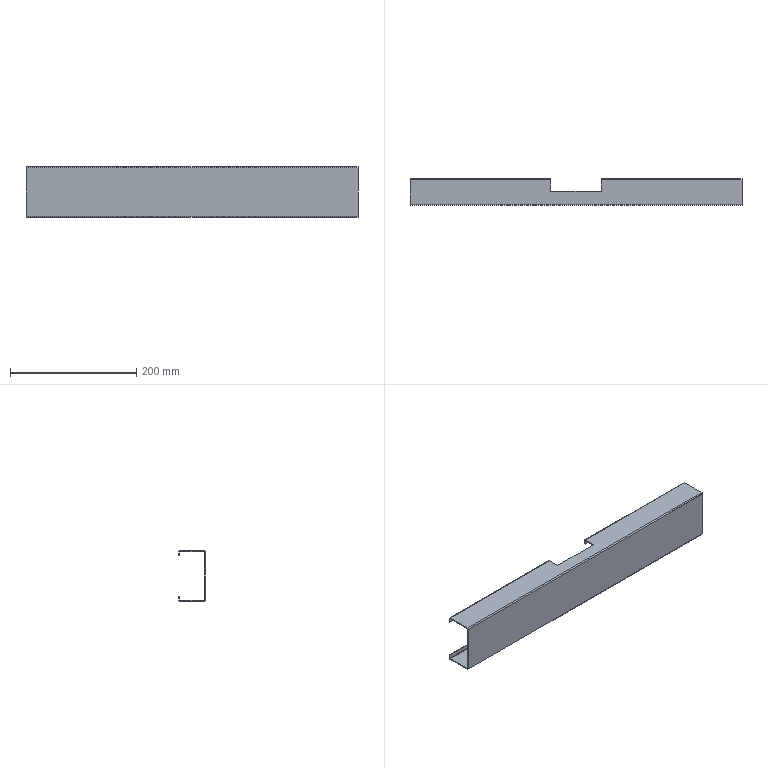Part | 1 solid | 62 faces | box 525 x 42 x 80 mm | volume 129478 mm3 | plane 50 | cylinder 12 | commonest cylinder face diameters 0.4 x6 3.4 x6
STEP:
#1=CARTESIAN_POINT('',(-40.,42.,38.3));
#2=VERTEX_POINT('',#1);
#3=CARTESIAN_POINT('',(-40.,42.,32.));
#4=VERTEX_POINT('',#3);
#5=CARTESIAN_POINT('',(-40.,42.,32.));
#6=DIRECTION('',(0.,0.,-1.));
#7=VECTOR('',#6,1000.);
#8=LINE('',#5,#7);
#9=EDGE_CURVE('',#2,#4,#8,.T.);
#10=ORIENTED_EDGE('',*,*,#9,.F.);
#11=CARTESIAN_POINT('',(-40.,40.5,38.3));
#12=VERTEX_POINT('',#11);
#13=CARTESIAN_POINT('',(-40.,42.,38.3));
#14=DIRECTION('',(0.,-1.,0.));
#15=VECTOR('',#14,1000.);
#16=LINE('',#13,#15);
#17=EDGE_CURVE('',#2,#12,#16,.T.);
#18=ORIENTED_EDGE('',*,*,#17,.T.);
#19=CARTESIAN_POINT('',(-40.,40.5,32.));
#20=VERTEX_POINT('',#19);
#21=CARTESIAN_POINT('',(-40.,40.5,32.));
#22=DIRECTION('',(0.,0.,-1.));
#23=VECTOR('',#22,1000.);
#24=LINE('',#21,#23);
#25=EDGE_CURVE('',#12,#20,#24,.T.);
#26=ORIENTED_EDGE('',*,*,#25,.T.);
#27=CARTESIAN_POINT('',(-40.,42.,32.));
#28=DIRECTION('',(0.,1.,0.));
#29=VECTOR('',#28,1000.);
#30=LINE('',#27,#29);
#31=EDGE_CURVE('',#20,#4,#30,.T.);
#32=ORIENTED_EDGE('',*,*,#31,.T.);
#33=EDGE_LOOP('',(#10,#18,#26,#32));
#34=FACE_OUTER_BOUND('',#33,.T.);
#35=CARTESIAN_POINT('',(-40.,62.,-40.));
#36=DIRECTION('',(-1.,0.,0.));
#37=DIRECTION('',(0.,0.,1.));
#38=AXIS2_PLACEMENT_3D('',#35,#36,#37);
#39=PLANE('',#38);
#40=ADVANCED_FACE('',(#34),#39,.F.);
#41=CARTESIAN_POINT('',(-40.,22.,38.5));
#42=VERTEX_POINT('',#41);
#43=CARTESIAN_POINT('',(-40.,40.3,38.5));
#44=VERTEX_POINT('',#43);
#45=CARTESIAN_POINT('',(-40.,42.,38.5));
#46=DIRECTION('',(0.,1.,0.));
#47=VECTOR('',#46,1000.);
#48=LINE('',#45,#47);
#49=EDGE_CURVE('',#42,#44,#48,.T.);
#50=ORIENTED_EDGE('',*,*,#49,.T.);
#51=CARTESIAN_POINT('',(-40.,40.3,40.));
#52=VERTEX_POINT('',#51);
#53=CARTESIAN_POINT('',(-40.,40.3,38.5));
#54=DIRECTION('',(0.,0.,1.));
#55=VECTOR('',#54,1000.);
#56=LINE('',#53,#55);
#57=EDGE_CURVE('',#44,#52,#56,.T.);
#58=ORIENTED_EDGE('',*,*,#57,.T.);
#59=CARTESIAN_POINT('',(-40.,22.,40.));
#60=VERTEX_POINT('',#59);
#61=CARTESIAN_POINT('',(-40.,42.,40.));
#62=DIRECTION('',(0.,1.,0.));
#63=VECTOR('',#62,1000.);
#64=LINE('',#61,#63);
#65=EDGE_CURVE('',#60,#52,#64,.T.);
#66=ORIENTED_EDGE('',*,*,#65,.F.);
#67=CARTESIAN_POINT('',(-40.,22.,-40.));
#68=DIRECTION('',(0.,0.,1.));
#69=VECTOR('',#68,1000.);
#70=LINE('',#67,#69);
#71=EDGE_CURVE('',#42,#60,#70,.T.);
#72=ORIENTED_EDGE('',*,*,#71,.F.);
#73=EDGE_LOOP('',(#50,#58,#66,#72));
#74=FACE_OUTER_BOUND('',#73,.T.);
#75=CARTESIAN_POINT('',(-40.,62.,-40.));
#76=DIRECTION('',(-1.,0.,0.));
#77=DIRECTION('',(0.,0.,1.));
#78=AXIS2_PLACEMENT_3D('',#75,#76,#77);
#79=PLANE('',#78);
#80=ADVANCED_FACE('',(#74),#79,.F.);
#81=CARTESIAN_POINT('',(40.,40.5,32.));
#82=VERTEX_POINT('',#81);
#83=CARTESIAN_POINT('',(40.,40.5,38.3));
#84=VERTEX_POINT('',#83);
#85=CARTESIAN_POINT('',(40.,40.5,32.));
#86=DIRECTION('',(0.,0.,1.));
#87=VECTOR('',#86,1000.);
#88=LINE('',#85,#87);
#89=EDGE_CURVE('',#82,#84,#88,.T.);
#90=ORIENTED_EDGE('',*,*,#89,.T.);
#91=CARTESIAN_POINT('',(40.,42.,38.3));
#92=VERTEX_POINT('',#91);
#93=CARTESIAN_POINT('',(40.,40.5,38.3));
#94=DIRECTION('',(0.,1.,0.));
#95=VECTOR('',#94,1000.);
#96=LINE('',#93,#95);
#97=EDGE_CURVE('',#84,#92,#96,.T.);
#98=ORIENTED_EDGE('',*,*,#97,.T.);
#99=CARTESIAN_POINT('',(40.,42.,32.));
#100=VERTEX_POINT('',#99);
#101=CARTESIAN_POINT('',(40.,42.,32.));
#102=DIRECTION('',(0.,0.,1.));
#103=VECTOR('',#102,1000.);
#104=LINE('',#101,#103);
#105=EDGE_CURVE('',#100,#92,#104,.T.);
#106=ORIENTED_EDGE('',*,*,#105,.F.);
#107=CARTESIAN_POINT('',(40.,42.,32.));
#108=DIRECTION('',(0.,-1.,0.));
#109=VECTOR('',#108,1000.);
#110=LINE('',#107,#109);
#111=EDGE_CURVE('',#100,#82,#110,.T.);
#112=ORIENTED_EDGE('',*,*,#111,.T.);
#113=EDGE_LOOP('',(#90,#98,#106,#112));
#114=FACE_OUTER_BOUND('',#113,.T.);
#115=CARTESIAN_POINT('',(40.,62.,-40.));
#116=DIRECTION('',(1.,0.,0.));
#117=DIRECTION('',(0.,0.,-1.));
#118=AXIS2_PLACEMENT_3D('',#115,#116,#117);
#119=PLANE('',#118);
#120=ADVANCED_FACE('',(#114),#119,.F.);
#121=CARTESIAN_POINT('',(40.,40.3,40.));
#122=VERTEX_POINT('',#121);
#123=CARTESIAN_POINT('',(40.,22.,40.));
#124=VERTEX_POINT('',#123);
#125=CARTESIAN_POINT('',(40.,42.,40.));
#126=DIRECTION('',(0.,-1.,0.));
#127=VECTOR('',#126,1000.);
#128=LINE('',#125,#127);
#129=EDGE_CURVE('',#122,#124,#128,.T.);
#130=ORIENTED_EDGE('',*,*,#129,.F.);
#131=CARTESIAN_POINT('',(40.,40.3,38.5));
#132=VERTEX_POINT('',#131);
#133=CARTESIAN_POINT('',(40.,40.3,40.));
#134=DIRECTION('',(0.,0.,-1.));
#135=VECTOR('',#134,1000.);
#136=LINE('',#133,#135);
#137=EDGE_CURVE('',#122,#132,#136,.T.);
#138=ORIENTED_EDGE('',*,*,#137,.T.);
#139=CARTESIAN_POINT('',(40.,22.,38.5));
#140=VERTEX_POINT('',#139);
#141=CARTESIAN_POINT('',(40.,42.,38.5));
#142=DIRECTION('',(0.,-1.,0.));
#143=VECTOR('',#142,1000.);
#144=LINE('',#141,#143);
#145=EDGE_CURVE('',#132,#140,#144,.T.);
#146=ORIENTED_EDGE('',*,*,#145,.T.);
#147=CARTESIAN_POINT('',(40.,22.,-40.));
#148=DIRECTION('',(0.,0.,1.));
#149=VECTOR('',#148,1000.);
#150=LINE('',#147,#149);
#151=EDGE_CURVE('',#140,#124,#150,.T.);
#152=ORIENTED_EDGE('',*,*,#151,.T.);
#153=EDGE_LOOP('',(#130,#138,#146,#152));
#154=FACE_OUTER_BOUND('',#153,.T.);
#155=CARTESIAN_POINT('',(40.,62.,-40.));
#156=DIRECTION('',(1.,0.,0.));
#157=DIRECTION('',(0.,0.,-1.));
#158=AXIS2_PLACEMENT_3D('',#155,#156,#157);
#159=PLANE('',#158);
#160=ADVANCED_FACE('',(#154),#159,.F.);
#161=CARTESIAN_POINT('',(-40.,40.5,-32.));
#162=VERTEX_POINT('',#161);
#163=CARTESIAN_POINT('',(-40.,40.5,-38.3));
#164=VERTEX_POINT('',#163);
#165=CARTESIAN_POINT('',(-40.,40.5,-40.));
#166=DIRECTION('',(0.,0.,-1.));
#167=VECTOR('',#166,1000.);
#168=LINE('',#165,#167);
#169=EDGE_CURVE('',#162,#164,#168,.T.);
#170=ORIENTED_EDGE('',*,*,#169,.T.);
#171=CARTESIAN_POINT('',(-40.,42.,-38.3));
#172=VERTEX_POINT('',#171);
#173=CARTESIAN_POINT('',(-40.,40.5,-38.3));
#174=DIRECTION('',(0.,1.,0.));
#175=VECTOR('',#174,1000.);
#176=LINE('',#173,#175);
#177=EDGE_CURVE('',#164,#172,#176,.T.);
#178=ORIENTED_EDGE('',*,*,#177,.T.);
#179=CARTESIAN_POINT('',(-40.,42.,-32.));
#180=VERTEX_POINT('',#179);
#181=CARTESIAN_POINT('',(-40.,42.,-40.));
#182=DIRECTION('',(0.,0.,-1.));
#183=VECTOR('',#182,1000.);
#184=LINE('',#181,#183);
#185=EDGE_CURVE('',#180,#172,#184,.T.);
#186=ORIENTED_EDGE('',*,*,#185,.F.);
#187=CARTESIAN_POINT('',(-40.,40.5,-32.));
#188=DIRECTION('',(0.,-1.,0.));
#189=VECTOR('',#188,1000.);
#190=LINE('',#187,#189);
#191=EDGE_CURVE('',#180,#162,#190,.T.);
#192=ORIENTED_EDGE('',*,*,#191,.T.);
#193=EDGE_LOOP('',(#170,#178,#186,#192));
#194=FACE_OUTER_BOUND('',#193,.T.);
#195=CARTESIAN_POINT('',(-40.,62.,-40.));
#196=DIRECTION('',(-1.,0.,0.));
#197=DIRECTION('',(0.,0.,1.));
#198=AXIS2_PLACEMENT_3D('',#195,#196,#197);
#199=PLANE('',#198);
#200=ADVANCED_FACE('',(#194),#199,.F.);
#201=CARTESIAN_POINT('',(-40.,40.3,-40.));
#202=VERTEX_POINT('',#201);
#203=CARTESIAN_POINT('',(-40.,22.,-40.));
#204=VERTEX_POINT('',#203);
#205=CARTESIAN_POINT('',(-40.,62.,-40.));
#206=DIRECTION('',(0.,-1.,0.));
#207=VECTOR('',#206,1000.);
#208=LINE('',#205,#207);
#209=EDGE_CURVE('',#202,#204,#208,.T.);
#210=ORIENTED_EDGE('',*,*,#209,.F.);
#211=CARTESIAN_POINT('',(-40.,40.3,-38.5));
#212=VERTEX_POINT('',#211);
#213=CARTESIAN_POINT('',(-40.,40.3,-40.));
#214=DIRECTION('',(0.,0.,1.));
#215=VECTOR('',#214,1000.);
#216=LINE('',#213,#215);
#217=EDGE_CURVE('',#202,#212,#216,.T.);
#218=ORIENTED_EDGE('',*,*,#217,.T.);
#219=CARTESIAN_POINT('',(-40.,22.,-38.5));
#220=VERTEX_POINT('',#219);
#221=CARTESIAN_POINT('',(-40.,0.,-38.5));
#222=DIRECTION('',(0.,-1.,0.));
#223=VECTOR('',#222,1000.);
#224=LINE('',#221,#223);
#225=EDGE_CURVE('',#212,#220,#224,.T.);
#226=ORIENTED_EDGE('',*,*,#225,.T.);
#227=CARTESIAN_POINT('',(-40.,22.,-40.));
#228=DIRECTION('',(0.,0.,1.));
#229=VECTOR('',#228,1000.);
#230=LINE('',#227,#229);
#231=EDGE_CURVE('',#204,#220,#230,.T.);
#232=ORIENTED_EDGE('',*,*,#231,.F.);
#233=EDGE_LOOP('',(#210,#218,#226,#232));
#234=FACE_OUTER_BOUND('',#233,.T.);
#235=CARTESIAN_POINT('',(-40.,62.,-40.));
#236=DIRECTION('',(-1.,0.,0.));
#237=DIRECTION('',(0.,0.,1.));
#238=AXIS2_PLACEMENT_3D('',#235,#236,#237);
#239=PLANE('',#238);
#240=ADVANCED_FACE('',(#234),#239,.F.);
#241=CARTESIAN_POINT('',(40.,42.,-38.3));
#242=VERTEX_POINT('',#241);
#243=CARTESIAN_POINT('',(40.,42.,-32.));
#244=VERTEX_POINT('',#243);
#245=CARTESIAN_POINT('',(40.,42.,-40.));
#246=DIRECTION('',(0.,0.,1.));
#247=VECTOR('',#246,1000.);
#248=LINE('',#245,#247);
#249=EDGE_CURVE('',#242,#244,#248,.T.);
#250=ORIENTED_EDGE('',*,*,#249,.F.);
#251=CARTESIAN_POINT('',(40.,40.5,-38.3));
#252=VERTEX_POINT('',#251);
#253=CARTESIAN_POINT('',(40.,42.,-38.3));
#254=DIRECTION('',(0.,-1.,0.));
#255=VECTOR('',#254,1000.);
#256=LINE('',#253,#255);
#257=EDGE_CURVE('',#242,#252,#256,.T.);
#258=ORIENTED_EDGE('',*,*,#257,.T.);
#259=CARTESIAN_POINT('',(40.,40.5,-32.));
#260=VERTEX_POINT('',#259);
#261=CARTESIAN_POINT('',(40.,40.5,-40.));
#262=DIRECTION('',(0.,0.,1.));
#263=VECTOR('',#262,1000.);
#264=LINE('',#261,#263);
#265=EDGE_CURVE('',#252,#260,#264,.T.);
#266=ORIENTED_EDGE('',*,*,#265,.T.);
#267=CARTESIAN_POINT('',(40.,40.5,-32.));
#268=DIRECTION('',(0.,1.,0.));
#269=VECTOR('',#268,1000.);
#270=LINE('',#267,#269);
#271=EDGE_CURVE('',#260,#244,#270,.T.);
#272=ORIENTED_EDGE('',*,*,#271,.T.);
#273=EDGE_LOOP('',(#250,#258,#266,#272));
#274=FACE_OUTER_BOUND('',#273,.T.);
#275=CARTESIAN_POINT('',(40.,62.,-40.));
#276=DIRECTION('',(1.,0.,0.));
#277=DIRECTION('',(0.,0.,-1.));
#278=AXIS2_PLACEMENT_3D('',#275,#276,#277);
#279=PLANE('',#278);
#280=ADVANCED_FACE('',(#274),#279,.F.);
#281=CARTESIAN_POINT('',(40.,22.,-38.5));
#282=VERTEX_POINT('',#281);
#283=CARTESIAN_POINT('',(40.,40.3,-38.5));
#284=VERTEX_POINT('',#283);
#285=CARTESIAN_POINT('',(40.,0.,-38.5));
#286=DIRECTION('',(0.,1.,0.));
#287=VECTOR('',#286,1000.);
#288=LINE('',#285,#287);
#289=EDGE_CURVE('',#282,#284,#288,.T.);
#290=ORIENTED_EDGE('',*,*,#289,.T.);
#291=CARTESIAN_POINT('',(40.,40.3,-40.));
#292=VERTEX_POINT('',#291);
#293=CARTESIAN_POINT('',(40.,40.3,-38.5));
#294=DIRECTION('',(0.,0.,-1.));
#295=VECTOR('',#294,1000.);
#296=LINE('',#293,#295);
#297=EDGE_CURVE('',#284,#292,#296,.T.);
#298=ORIENTED_EDGE('',*,*,#297,.T.);
#299=CARTESIAN_POINT('',(40.,22.,-40.));
#300=VERTEX_POINT('',#299);
#301=CARTESIAN_POINT('',(40.,62.,-40.));
#302=DIRECTION('',(0.,1.,0.));
#303=VECTOR('',#302,1000.);
#304=LINE('',#301,#303);
#305=EDGE_CURVE('',#300,#292,#304,.T.);
#306=ORIENTED_EDGE('',*,*,#305,.F.);
#307=CARTESIAN_POINT('',(40.,22.,-40.));
#308=DIRECTION('',(0.,0.,1.));
#309=VECTOR('',#308,1000.);
#310=LINE('',#307,#309);
#311=EDGE_CURVE('',#300,#282,#310,.T.);
#312=ORIENTED_EDGE('',*,*,#311,.T.);
#313=EDGE_LOOP('',(#290,#298,#306,#312));
#314=FACE_OUTER_BOUND('',#313,.T.);
#315=CARTESIAN_POINT('',(40.,62.,-40.));
#316=DIRECTION('',(1.,0.,0.));
#317=DIRECTION('',(0.,0.,-1.));
#318=AXIS2_PLACEMENT_3D('',#315,#316,#317);
#319=PLANE('',#318);
#320=ADVANCED_FACE('',(#314),#319,.F.);
#321=CARTESIAN_POINT('',(262.5,42.,-38.3));
#322=VERTEX_POINT('',#321);
#323=CARTESIAN_POINT('',(262.5,42.,-38.3));
#324=DIRECTION('',(-1.,0.,0.));
#325=VECTOR('',#324,1000.);
#326=LINE('',#323,#325);
#327=EDGE_CURVE('',#322,#242,#326,.T.);
#328=ORIENTED_EDGE('',*,*,#327,.T.);
#329=ORIENTED_EDGE('',*,*,#249,.T.);
#330=CARTESIAN_POINT('',(262.5,42.,-32.));
#331=VERTEX_POINT('',#330);
#332=CARTESIAN_POINT('',(262.5,42.,-32.));
#333=DIRECTION('',(-1.,0.,0.));
#334=VECTOR('',#333,1000.);
#335=LINE('',#332,#334);
#336=EDGE_CURVE('',#331,#244,#335,.T.);
#337=ORIENTED_EDGE('',*,*,#336,.F.);
#338=CARTESIAN_POINT('',(262.5,42.,-40.));
#339=DIRECTION('',(0.,0.,1.));
#340=VECTOR('',#339,1000.);
#341=LINE('',#338,#340);
#342=EDGE_CURVE('',#322,#331,#341,.T.);
#343=ORIENTED_EDGE('',*,*,#342,.F.);
#344=EDGE_LOOP('',(#328,#329,#337,#343));
#345=FACE_OUTER_BOUND('',#344,.T.);
#346=CARTESIAN_POINT('',(262.5,42.,-40.));
#347=DIRECTION('',(0.,-1.,0.));
#348=DIRECTION('',(0.,0.,-1.));
#349=AXIS2_PLACEMENT_3D('',#346,#347,#348);
#350=PLANE('',#349);
#351=ADVANCED_FACE('',(#345),#350,.F.);
#352=ORIENTED_EDGE('',*,*,#271,.F.);
#353=CARTESIAN_POINT('',(262.5,40.5,-32.));
#354=VERTEX_POINT('',#353);
#355=CARTESIAN_POINT('',(262.5,40.5,-32.));
#356=DIRECTION('',(-1.,0.,0.));
#357=VECTOR('',#356,1000.);
#358=LINE('',#355,#357);
#359=EDGE_CURVE('',#354,#260,#358,.T.);
#360=ORIENTED_EDGE('',*,*,#359,.F.);
#361=CARTESIAN_POINT('',(262.5,40.5,-32.));
#362=DIRECTION('',(0.,1.,0.));
#363=VECTOR('',#362,1000.);
#364=LINE('',#361,#363);
#365=EDGE_CURVE('',#354,#331,#364,.T.);
#366=ORIENTED_EDGE('',*,*,#365,.T.);
#367=ORIENTED_EDGE('',*,*,#336,.T.);
#368=EDGE_LOOP('',(#352,#360,#366,#367));
#369=FACE_OUTER_BOUND('',#368,.T.);
#370=CARTESIAN_POINT('',(262.5,40.5,-32.));
#371=DIRECTION('',(0.,0.,1.));
#372=DIRECTION('',(1.,0.,0.));
#373=AXIS2_PLACEMENT_3D('',#370,#371,#372);
#374=PLANE('',#373);
#375=ADVANCED_FACE('',(#369),#374,.T.);
#376=ORIENTED_EDGE('',*,*,#265,.F.);
#377=CARTESIAN_POINT('',(262.5,40.5,-38.3));
#378=VERTEX_POINT('',#377);
#379=CARTESIAN_POINT('',(262.5,40.5,-38.3));
#380=DIRECTION('',(-1.,0.,0.));
#381=VECTOR('',#380,1000.);
#382=LINE('',#379,#381);
#383=EDGE_CURVE('',#378,#252,#382,.T.);
#384=ORIENTED_EDGE('',*,*,#383,.F.);
#385=CARTESIAN_POINT('',(262.5,40.5,-40.));
#386=DIRECTION('',(0.,0.,1.));
#387=VECTOR('',#386,1000.);
#388=LINE('',#385,#387);
#389=EDGE_CURVE('',#378,#354,#388,.T.);
#390=ORIENTED_EDGE('',*,*,#389,.T.);
#391=ORIENTED_EDGE('',*,*,#359,.T.);
#392=EDGE_LOOP('',(#376,#384,#390,#391));
#393=FACE_OUTER_BOUND('',#392,.T.);
#394=CARTESIAN_POINT('',(262.5,40.5,-40.));
#395=DIRECTION('',(0.,-1.,0.));
#396=DIRECTION('',(0.,0.,-1.));
#397=AXIS2_PLACEMENT_3D('',#394,#395,#396);
#398=PLANE('',#397);
#399=ADVANCED_FACE('',(#393),#398,.T.);
#400=CARTESIAN_POINT('',(40.,40.3,-38.3));
#401=DIRECTION('',(1.,0.,0.));
#402=DIRECTION('',(0.,0.,-1.));
#403=AXIS2_PLACEMENT_3D('',#400,#401,#402);
#404=CIRCLE('',#403,0.2);
#405=EDGE_CURVE('',#284,#252,#404,.T.);
#406=ORIENTED_EDGE('',*,*,#405,.F.);
#407=CARTESIAN_POINT('',(262.5,40.3,-38.5));
#408=VERTEX_POINT('',#407);
#409=CARTESIAN_POINT('',(262.5,40.3,-38.5));
#410=DIRECTION('',(-1.,0.,0.));
#411=VECTOR('',#410,1000.);
#412=LINE('',#409,#411);
#413=EDGE_CURVE('',#408,#284,#412,.T.);
#414=ORIENTED_EDGE('',*,*,#413,.F.);
#415=CARTESIAN_POINT('',(262.5,40.3,-38.3));
#416=DIRECTION('',(1.,0.,0.));
#417=DIRECTION('',(0.,0.,-1.));
#418=AXIS2_PLACEMENT_3D('',#415,#416,#417);
#419=CIRCLE('',#418,0.2);
#420=EDGE_CURVE('',#408,#378,#419,.T.);
#421=ORIENTED_EDGE('',*,*,#420,.T.);
#422=ORIENTED_EDGE('',*,*,#383,.T.);
#423=EDGE_LOOP('',(#406,#414,#421,#422));
#424=FACE_OUTER_BOUND('',#423,.T.);
#425=CARTESIAN_POINT('',(262.5,40.3,-38.3));
#426=DIRECTION('',(-1.,0.,0.));
#427=DIRECTION('',(0.,0.,1.));
#428=AXIS2_PLACEMENT_3D('',#425,#426,#427);
#429=CYLINDRICAL_SURFACE('',#428,0.2);
#430=ADVANCED_FACE('',(#424),#429,.F.);
#431=CARTESIAN_POINT('',(40.,40.3,38.3));
#432=DIRECTION('',(1.,0.,0.));
#433=DIRECTION('',(0.,0.,-1.));
#434=AXIS2_PLACEMENT_3D('',#431,#432,#433);
#435=CIRCLE('',#434,0.2);
#436=EDGE_CURVE('',#84,#132,#435,.T.);
#437=ORIENTED_EDGE('',*,*,#436,.F.);
#438=CARTESIAN_POINT('',(262.5,40.5,38.3));
#439=VERTEX_POINT('',#438);
#440=CARTESIAN_POINT('',(262.5,40.5,38.3));
#441=DIRECTION('',(-1.,0.,0.));
#442=VECTOR('',#441,1000.);
#443=LINE('',#440,#442);
#444=EDGE_CURVE('',#439,#84,#443,.T.);
#445=ORIENTED_EDGE('',*,*,#444,.F.);
#446=CARTESIAN_POINT('',(262.5,40.3,38.5));
#447=VERTEX_POINT('',#446);
#448=CARTESIAN_POINT('',(262.5,40.3,38.3));
#449=DIRECTION('',(1.,0.,0.));
#450=DIRECTION('',(0.,0.,-1.));
#451=AXIS2_PLACEMENT_3D('',#448,#449,#450);
#452=CIRCLE('',#451,0.2);
#453=EDGE_CURVE('',#439,#447,#452,.T.);
#454=ORIENTED_EDGE('',*,*,#453,.T.);
#455=CARTESIAN_POINT('',(262.5,40.3,38.5));
#456=DIRECTION('',(-1.,0.,0.));
#457=VECTOR('',#456,1000.);
#458=LINE('',#455,#457);
#459=EDGE_CURVE('',#447,#132,#458,.T.);
#460=ORIENTED_EDGE('',*,*,#459,.T.);
#461=EDGE_LOOP('',(#437,#445,#454,#460));
#462=FACE_OUTER_BOUND('',#461,.T.);
#463=CARTESIAN_POINT('',(262.5,40.3,38.3));
#464=DIRECTION('',(-1.,0.,0.));
#465=DIRECTION('',(0.,0.,1.));
#466=AXIS2_PLACEMENT_3D('',#463,#464,#465);
#467=CYLINDRICAL_SURFACE('',#466,0.2);
#468=ADVANCED_FACE('',(#462),#467,.F.);
#469=ORIENTED_EDGE('',*,*,#89,.F.);
#470=CARTESIAN_POINT('',(262.5,40.5,32.));
#471=VERTEX_POINT('',#470);
#472=CARTESIAN_POINT('',(262.5,40.5,32.));
#473=DIRECTION('',(-1.,0.,0.));
#474=VECTOR('',#473,1000.);
#475=LINE('',#472,#474);
#476=EDGE_CURVE('',#471,#82,#475,.T.);
#477=ORIENTED_EDGE('',*,*,#476,.F.);
#478=CARTESIAN_POINT('',(262.5,40.5,32.));
#479=DIRECTION('',(0.,0.,1.));
#480=VECTOR('',#479,1000.);
#481=LINE('',#478,#480);
#482=EDGE_CURVE('',#471,#439,#481,.T.);
#483=ORIENTED_EDGE('',*,*,#482,.T.);
#484=ORIENTED_EDGE('',*,*,#444,.T.);
#485=EDGE_LOOP('',(#469,#477,#483,#484));
#486=FACE_OUTER_BOUND('',#485,.T.);
#487=CARTESIAN_POINT('',(262.5,40.5,32.));
#488=DIRECTION('',(0.,-1.,0.));
#489=DIRECTION('',(0.,0.,-1.));
#490=AXIS2_PLACEMENT_3D('',#487,#488,#489);
#491=PLANE('',#490);
#492=ADVANCED_FACE('',(#486),#491,.T.);
#493=ORIENTED_EDGE('',*,*,#111,.F.);
#494=CARTESIAN_POINT('',(262.5,42.,32.));
#495=VERTEX_POINT('',#494);
#496=CARTESIAN_POINT('',(262.5,42.,32.));
#497=DIRECTION('',(-1.,0.,0.));
#498=VECTOR('',#497,1000.);
#499=LINE('',#496,#498);
#500=EDGE_CURVE('',#495,#100,#499,.T.);
#501=ORIENTED_EDGE('',*,*,#500,.F.);
#502=CARTESIAN_POINT('',(262.5,42.,32.));
#503=DIRECTION('',(0.,-1.,0.));
#504=VECTOR('',#503,1000.);
#505=LINE('',#502,#504);
#506=EDGE_CURVE('',#495,#471,#505,.T.);
#507=ORIENTED_EDGE('',*,*,#506,.T.);
#508=ORIENTED_EDGE('',*,*,#476,.T.);
#509=EDGE_LOOP('',(#493,#501,#507,#508));
#510=FACE_OUTER_BOUND('',#509,.T.);
#511=CARTESIAN_POINT('',(262.5,42.,32.));
#512=DIRECTION('',(0.,0.,-1.));
#513=DIRECTION('',(-1.,0.,0.));
#514=AXIS2_PLACEMENT_3D('',#511,#512,#513);
#515=PLANE('',#514);
#516=ADVANCED_FACE('',(#510),#515,.T.);
#517=ORIENTED_EDGE('',*,*,#500,.T.);
#518=ORIENTED_EDGE('',*,*,#105,.T.);
#519=CARTESIAN_POINT('',(262.5,42.,38.3));
#520=VERTEX_POINT('',#519);
#521=CARTESIAN_POINT('',(262.5,42.,38.3));
#522=DIRECTION('',(-1.,0.,0.));
#523=VECTOR('',#522,1000.);
#524=LINE('',#521,#523);
#525=EDGE_CURVE('',#520,#92,#524,.T.);
#526=ORIENTED_EDGE('',*,*,#525,.F.);
#527=CARTESIAN_POINT('',(262.5,42.,32.));
#528=DIRECTION('',(0.,0.,1.));
#529=VECTOR('',#528,1000.);
#530=LINE('',#527,#529);
#531=EDGE_CURVE('',#495,#520,#530,.T.);
#532=ORIENTED_EDGE('',*,*,#531,.F.);
#533=EDGE_LOOP('',(#517,#518,#526,#532));
#534=FACE_OUTER_BOUND('',#533,.T.);
#535=CARTESIAN_POINT('',(262.5,42.,32.));
#536=DIRECTION('',(0.,-1.,0.));
#537=DIRECTION('',(0.,0.,-1.));
#538=AXIS2_PLACEMENT_3D('',#535,#536,#537);
#539=PLANE('',#538);
#540=ADVANCED_FACE('',(#534),#539,.F.);
#541=ORIENTED_EDGE('',*,*,#525,.T.);
#542=CARTESIAN_POINT('',(40.,40.3,38.3));
#543=DIRECTION('',(1.,0.,0.));
#544=DIRECTION('',(0.,0.,-1.));
#545=AXIS2_PLACEMENT_3D('',#542,#543,#544);
#546=CIRCLE('',#545,1.7);
#547=EDGE_CURVE('',#92,#122,#546,.T.);
#548=ORIENTED_EDGE('',*,*,#547,.T.);
#549=CARTESIAN_POINT('',(262.5,40.3,40.));
#550=VERTEX_POINT('',#549);
#551=CARTESIAN_POINT('',(262.5,40.3,40.));
#552=DIRECTION('',(-1.,0.,0.));
#553=VECTOR('',#552,1000.);
#554=LINE('',#551,#553);
#555=EDGE_CURVE('',#550,#122,#554,.T.);
#556=ORIENTED_EDGE('',*,*,#555,.F.);
#557=CARTESIAN_POINT('',(262.5,40.3,38.3));
#558=DIRECTION('',(1.,0.,0.));
#559=DIRECTION('',(0.,0.,1.));
#560=AXIS2_PLACEMENT_3D('',#557,#558,#559);
#561=CIRCLE('',#560,1.7);
#562=EDGE_CURVE('',#520,#550,#561,.T.);
#563=ORIENTED_EDGE('',*,*,#562,.F.);
#564=EDGE_LOOP('',(#541,#548,#556,#563));
#565=FACE_OUTER_BOUND('',#564,.T.);
#566=CARTESIAN_POINT('',(262.5,40.3,38.3));
#567=DIRECTION('',(-1.,0.,0.));
#568=DIRECTION('',(0.,0.,1.));
#569=AXIS2_PLACEMENT_3D('',#566,#567,#568);
#570=CYLINDRICAL_SURFACE('',#569,1.7);
#571=ADVANCED_FACE('',(#565),#570,.T.);
#572=CARTESIAN_POINT('',(262.5,40.3,-40.));
#573=VERTEX_POINT('',#572);
#574=CARTESIAN_POINT('',(262.5,40.3,-40.));
#575=DIRECTION('',(-1.,0.,0.));
#576=VECTOR('',#575,1000.);
#577=LINE('',#574,#576);
#578=EDGE_CURVE('',#573,#292,#577,.T.);
#579=ORIENTED_EDGE('',*,*,#578,.T.);
#580=CARTESIAN_POINT('',(40.,40.3,-38.3));
#581=DIRECTION('',(1.,0.,0.));
#582=DIRECTION('',(0.,0.,-1.));
#583=AXIS2_PLACEMENT_3D('',#580,#581,#582);
#584=CIRCLE('',#583,1.7);
#585=EDGE_CURVE('',#292,#242,#584,.T.);
#586=ORIENTED_EDGE('',*,*,#585,.T.);
#587=ORIENTED_EDGE('',*,*,#327,.F.);
#588=CARTESIAN_POINT('',(262.5,40.3,-38.3));
#589=DIRECTION('',(1.,0.,0.));
#590=DIRECTION('',(0.,0.,1.));
#591=AXIS2_PLACEMENT_3D('',#588,#589,#590);
#592=CIRCLE('',#591,1.7);
#593=EDGE_CURVE('',#573,#322,#592,.T.);
#594=ORIENTED_EDGE('',*,*,#593,.F.);
#595=EDGE_LOOP('',(#579,#586,#587,#594));
#596=FACE_OUTER_BOUND('',#595,.T.);
#597=CARTESIAN_POINT('',(262.5,40.3,-38.3));
#598=DIRECTION('',(-1.,0.,0.));
#599=DIRECTION('',(0.,0.,1.));
#600=AXIS2_PLACEMENT_3D('',#597,#598,#599);
#601=CYLINDRICAL_SURFACE('',#600,1.7);
#602=ADVANCED_FACE('',(#596),#601,.T.);
#603=CARTESIAN_POINT('',(262.5,42.,38.3));
#604=DIRECTION('',(0.,-1.,0.));
#605=VECTOR('',#604,1000.);
#606=LINE('',#603,#605);
#607=EDGE_CURVE('',#520,#439,#606,.T.);
#608=ORIENTED_EDGE('',*,*,#607,.F.);
#609=ORIENTED_EDGE('',*,*,#562,.T.);
#610=CARTESIAN_POINT('',(262.5,40.3,38.5));
#611=DIRECTION('',(0.,0.,1.));
#612=VECTOR('',#611,1000.);
#613=LINE('',#610,#612);
#614=EDGE_CURVE('',#447,#550,#613,.T.);
#615=ORIENTED_EDGE('',*,*,#614,.F.);
#616=ORIENTED_EDGE('',*,*,#453,.F.);
#617=EDGE_LOOP('',(#608,#609,#615,#616));
#618=FACE_OUTER_BOUND('',#617,.T.);
#619=CARTESIAN_POINT('',(262.5,42.,38.3));
#620=DIRECTION('',(1.,0.,0.));
#621=DIRECTION('',(0.,0.,-1.));
#622=AXIS2_PLACEMENT_3D('',#619,#620,#621);
#623=PLANE('',#622);
#624=ADVANCED_FACE('',(#618),#623,.T.);
#625=ORIENTED_EDGE('',*,*,#531,.T.);
#626=ORIENTED_EDGE('',*,*,#607,.T.);
#627=ORIENTED_EDGE('',*,*,#482,.F.);
#628=ORIENTED_EDGE('',*,*,#506,.F.);
#629=EDGE_LOOP('',(#625,#626,#627,#628));
#630=FACE_OUTER_BOUND('',#629,.T.);
#631=CARTESIAN_POINT('',(262.5,40.3,38.5));
#632=DIRECTION('',(1.,0.,0.));
#633=DIRECTION('',(0.,0.,-1.));
#634=AXIS2_PLACEMENT_3D('',#631,#632,#633);
#635=PLANE('',#634);
#636=ADVANCED_FACE('',(#630),#635,.T.);
#637=CARTESIAN_POINT('',(-262.5,40.3,40.));
#638=VERTEX_POINT('',#637);
#639=CARTESIAN_POINT('',(-262.5,40.3,38.5));
#640=VERTEX_POINT('',#639);
#641=CARTESIAN_POINT('',(-262.5,40.3,40.));
#642=DIRECTION('',(0.,0.,-1.));
#643=VECTOR('',#642,1000.);
#644=LINE('',#641,#643);
#645=EDGE_CURVE('',#638,#640,#644,.T.);
#646=ORIENTED_EDGE('',*,*,#645,.F.);
#647=CARTESIAN_POINT('',(-262.5,42.,38.3));
#648=VERTEX_POINT('',#647);
#649=CARTESIAN_POINT('',(-262.5,40.3,38.3));
#650=DIRECTION('',(1.,0.,0.));
#651=DIRECTION('',(0.,0.,1.));
#652=AXIS2_PLACEMENT_3D('',#649,#650,#651);
#653=CIRCLE('',#652,1.7);
#654=EDGE_CURVE('',#648,#638,#653,.T.);
#655=ORIENTED_EDGE('',*,*,#654,.F.);
#656=CARTESIAN_POINT('',(-262.5,40.5,38.3));
#657=VERTEX_POINT('',#656);
#658=CARTESIAN_POINT('',(-262.5,40.5,38.3));
#659=DIRECTION('',(0.,1.,0.));
#660=VECTOR('',#659,1000.);
#661=LINE('',#658,#660);
#662=EDGE_CURVE('',#657,#648,#661,.T.);
#663=ORIENTED_EDGE('',*,*,#662,.F.);
#664=CARTESIAN_POINT('',(-262.5,40.3,38.3));
#665=DIRECTION('',(1.,0.,0.));
#666=DIRECTION('',(0.,0.,-1.));
#667=AXIS2_PLACEMENT_3D('',#664,#665,#666);
#668=CIRCLE('',#667,0.2);
#669=EDGE_CURVE('',#657,#640,#668,.T.);
#670=ORIENTED_EDGE('',*,*,#669,.T.);
#671=EDGE_LOOP('',(#646,#655,#663,#670));
#672=FACE_OUTER_BOUND('',#671,.T.);
#673=CARTESIAN_POINT('',(-262.5,40.3,40.));
#674=DIRECTION('',(-1.,0.,0.));
#675=DIRECTION('',(0.,0.,1.));
#676=AXIS2_PLACEMENT_3D('',#673,#674,#675);
#677=PLANE('',#676);
#678=ADVANCED_FACE('',(#672),#677,.T.);
#679=CARTESIAN_POINT('',(-262.5,1.7,40.));
#680=VERTEX_POINT('',#679);
#681=CARTESIAN_POINT('',(-262.5,42.,40.));
#682=DIRECTION('',(0.,-1.,0.));
#683=VECTOR('',#682,1000.);
#684=LINE('',#681,#683);
#685=EDGE_CURVE('',#638,#680,#684,.T.);
#686=ORIENTED_EDGE('',*,*,#685,.F.);
#687=ORIENTED_EDGE('',*,*,#645,.T.);
#688=CARTESIAN_POINT('',(-262.5,1.7,38.5));
#689=VERTEX_POINT('',#688);
#690=CARTESIAN_POINT('',(-262.5,42.,38.5));
#691=DIRECTION('',(0.,-1.,0.));
#692=VECTOR('',#691,1000.);
#693=LINE('',#690,#692);
#694=EDGE_CURVE('',#640,#689,#693,.T.);
#695=ORIENTED_EDGE('',*,*,#694,.T.);
#696=CARTESIAN_POINT('',(-262.5,1.7,38.5));
#697=DIRECTION('',(0.,0.,1.));
#698=VECTOR('',#697,1000.);
#699=LINE('',#696,#698);
#700=EDGE_CURVE('',#689,#680,#699,.T.);
#701=ORIENTED_EDGE('',*,*,#700,.T.);
#702=EDGE_LOOP('',(#686,#687,#695,#701));
#703=FACE_OUTER_BOUND('',#702,.T.);
#704=CARTESIAN_POINT('',(-262.5,40.5,38.3));
#705=DIRECTION('',(-1.,0.,0.));
#706=DIRECTION('',(0.,0.,1.));
#707=AXIS2_PLACEMENT_3D('',#704,#705,#706);
#708=PLANE('',#707);
#709=ADVANCED_FACE('',(#703),#708,.T.);
#710=CARTESIAN_POINT('',(262.5,1.7,40.));
#711=VERTEX_POINT('',#710);
#712=CARTESIAN_POINT('',(262.5,1.7,38.5));
#713=VERTEX_POINT('',#712);
#714=CARTESIAN_POINT('',(262.5,1.7,40.));
#715=DIRECTION('',(0.,0.,-1.));
#716=VECTOR('',#715,1000.);
#717=LINE('',#714,#716);
#718=EDGE_CURVE('',#711,#713,#717,.T.);
#719=ORIENTED_EDGE('',*,*,#718,.F.);
#720=CARTESIAN_POINT('',(262.5,0.,38.3));
#721=VERTEX_POINT('',#720);
#722=CARTESIAN_POINT('',(262.5,1.7,38.3));
#723=DIRECTION('',(1.,0.,0.));
#724=DIRECTION('',(0.,0.,1.));
#725=AXIS2_PLACEMENT_3D('',#722,#723,#724);
#726=CIRCLE('',#725,1.7);
#727=EDGE_CURVE('',#711,#721,#726,.T.);
#728=ORIENTED_EDGE('',*,*,#727,.T.);
#729=CARTESIAN_POINT('',(262.5,1.5,38.3));
#730=VERTEX_POINT('',#729);
#731=CARTESIAN_POINT('',(262.5,1.5,38.3));
#732=DIRECTION('',(0.,-1.,0.));
#733=VECTOR('',#732,1000.);
#734=LINE('',#731,#733);
#735=EDGE_CURVE('',#730,#721,#734,.T.);
#736=ORIENTED_EDGE('',*,*,#735,.F.);
#737=CARTESIAN_POINT('',(262.5,1.7,38.3));
#738=DIRECTION('',(1.,0.,0.));
#739=DIRECTION('',(0.,0.,-1.));
#740=AXIS2_PLACEMENT_3D('',#737,#738,#739);
#741=CIRCLE('',#740,0.2);
#742=EDGE_CURVE('',#713,#730,#741,.T.);
#743=ORIENTED_EDGE('',*,*,#742,.F.);
#744=EDGE_LOOP('',(#719,#728,#736,#743));
#745=FACE_OUTER_BOUND('',#744,.T.);
#746=CARTESIAN_POINT('',(262.5,1.7,40.));
#747=DIRECTION('',(1.,0.,0.));
#748=DIRECTION('',(0.,0.,-1.));
#749=AXIS2_PLACEMENT_3D('',#746,#747,#748);
#750=PLANE('',#749);
#751=ADVANCED_FACE('',(#745),#750,.T.);
#752=CARTESIAN_POINT('',(262.5,42.,40.));
#753=DIRECTION('',(0.,-1.,0.));
#754=VECTOR('',#753,1000.);
#755=LINE('',#752,#754);
#756=EDGE_CURVE('',#550,#711,#755,.T.);
#757=ORIENTED_EDGE('',*,*,#756,.T.);
#758=ORIENTED_EDGE('',*,*,#718,.T.);
#759=CARTESIAN_POINT('',(262.5,42.,38.5));
#760=DIRECTION('',(0.,-1.,0.));
#761=VECTOR('',#760,1000.);
#762=LINE('',#759,#761);
#763=EDGE_CURVE('',#447,#713,#762,.T.);
#764=ORIENTED_EDGE('',*,*,#763,.F.);
#765=ORIENTED_EDGE('',*,*,#614,.T.);
#766=EDGE_LOOP('',(#757,#758,#764,#765));
#767=FACE_OUTER_BOUND('',#766,.T.);
#768=CARTESIAN_POINT('',(262.5,1.5,38.3));
#769=DIRECTION('',(1.,0.,0.));
#770=DIRECTION('',(0.,0.,-1.));
#771=AXIS2_PLACEMENT_3D('',#768,#769,#770);
#772=PLANE('',#771);
#773=ADVANCED_FACE('',(#767),#772,.T.);
#774=CARTESIAN_POINT('',(-262.5,0.,38.3));
#775=VERTEX_POINT('',#774);
#776=CARTESIAN_POINT('',(-262.5,1.5,38.3));
#777=VERTEX_POINT('',#776);
#778=CARTESIAN_POINT('',(-262.5,0.,38.3));
#779=DIRECTION('',(0.,1.,0.));
#780=VECTOR('',#779,1000.);
#781=LINE('',#778,#780);
#782=EDGE_CURVE('',#775,#777,#781,.T.);
#783=ORIENTED_EDGE('',*,*,#782,.F.);
#784=CARTESIAN_POINT('',(-262.5,1.7,38.3));
#785=DIRECTION('',(1.,0.,0.));
#786=DIRECTION('',(0.,0.,1.));
#787=AXIS2_PLACEMENT_3D('',#784,#785,#786);
#788=CIRCLE('',#787,1.7);
#789=EDGE_CURVE('',#680,#775,#788,.T.);
#790=ORIENTED_EDGE('',*,*,#789,.F.);
#791=ORIENTED_EDGE('',*,*,#700,.F.);
#792=CARTESIAN_POINT('',(-262.5,1.7,38.3));
#793=DIRECTION('',(1.,0.,0.));
#794=DIRECTION('',(0.,0.,-1.));
#795=AXIS2_PLACEMENT_3D('',#792,#793,#794);
#796=CIRCLE('',#795,0.2);
#797=EDGE_CURVE('',#689,#777,#796,.T.);
#798=ORIENTED_EDGE('',*,*,#797,.T.);
#799=EDGE_LOOP('',(#783,#790,#791,#798));
#800=FACE_OUTER_BOUND('',#799,.T.);
#801=CARTESIAN_POINT('',(-262.5,0.,38.3));
#802=DIRECTION('',(-1.,0.,0.));
#803=DIRECTION('',(0.,0.,1.));
#804=AXIS2_PLACEMENT_3D('',#801,#802,#803);
#805=PLANE('',#804);
#806=ADVANCED_FACE('',(#800),#805,.T.);
#807=CARTESIAN_POINT('',(-262.5,0.,-38.3));
#808=VERTEX_POINT('',#807);
#809=CARTESIAN_POINT('',(-262.5,0.,40.));
#810=DIRECTION('',(0.,0.,-1.));
#811=VECTOR('',#810,1000.);
#812=LINE('',#809,#811);
#813=EDGE_CURVE('',#775,#808,#812,.T.);
#814=ORIENTED_EDGE('',*,*,#813,.F.);
#815=ORIENTED_EDGE('',*,*,#782,.T.);
#816=CARTESIAN_POINT('',(-262.5,1.5,-38.3));
#817=VERTEX_POINT('',#816);
#818=CARTESIAN_POINT('',(-262.5,1.5,40.));
#819=DIRECTION('',(0.,0.,-1.));
#820=VECTOR('',#819,1000.);
#821=LINE('',#818,#820);
#822=EDGE_CURVE('',#777,#817,#821,.T.);
#823=ORIENTED_EDGE('',*,*,#822,.T.);
#824=CARTESIAN_POINT('',(-262.5,1.5,-38.3));
#825=DIRECTION('',(0.,-1.,0.));
#826=VECTOR('',#825,1000.);
#827=LINE('',#824,#826);
#828=EDGE_CURVE('',#817,#808,#827,.T.);
#829=ORIENTED_EDGE('',*,*,#828,.T.);
#830=EDGE_LOOP('',(#814,#815,#823,#829));
#831=FACE_OUTER_BOUND('',#830,.T.);
#832=CARTESIAN_POINT('',(-262.5,1.7,38.5));
#833=DIRECTION('',(-1.,0.,0.));
#834=DIRECTION('',(0.,0.,1.));
#835=AXIS2_PLACEMENT_3D('',#832,#833,#834);
#836=PLANE('',#835);
#837=ADVANCED_FACE('',(#831),#836,.T.);
#838=CARTESIAN_POINT('',(262.5,0.,-38.3));
#839=VERTEX_POINT('',#838);
#840=CARTESIAN_POINT('',(262.5,1.5,-38.3));
#841=VERTEX_POINT('',#840);
#842=CARTESIAN_POINT('',(262.5,0.,-38.3));
#843=DIRECTION('',(0.,1.,0.));
#844=VECTOR('',#843,1000.);
#845=LINE('',#842,#844);
#846=EDGE_CURVE('',#839,#841,#845,.T.);
#847=ORIENTED_EDGE('',*,*,#846,.F.);
#848=CARTESIAN_POINT('',(262.5,1.7,-40.));
#849=VERTEX_POINT('',#848);
#850=CARTESIAN_POINT('',(262.5,1.7,-38.3));
#851=DIRECTION('',(1.,0.,0.));
#852=DIRECTION('',(0.,0.,1.));
#853=AXIS2_PLACEMENT_3D('',#850,#851,#852);
#854=CIRCLE('',#853,1.7);
#855=EDGE_CURVE('',#839,#849,#854,.T.);
#856=ORIENTED_EDGE('',*,*,#855,.T.);
#857=CARTESIAN_POINT('',(262.5,1.7,-38.5));
#858=VERTEX_POINT('',#857);
#859=CARTESIAN_POINT('',(262.5,1.7,-38.5));
#860=DIRECTION('',(0.,0.,-1.));
#861=VECTOR('',#860,1000.);
#862=LINE('',#859,#861);
#863=EDGE_CURVE('',#858,#849,#862,.T.);
#864=ORIENTED_EDGE('',*,*,#863,.F.);
#865=CARTESIAN_POINT('',(262.5,1.7,-38.3));
#866=DIRECTION('',(1.,0.,0.));
#867=DIRECTION('',(0.,0.,-1.));
#868=AXIS2_PLACEMENT_3D('',#865,#866,#867);
#869=CIRCLE('',#868,0.2);
#870=EDGE_CURVE('',#841,#858,#869,.T.);
#871=ORIENTED_EDGE('',*,*,#870,.F.);
#872=EDGE_LOOP('',(#847,#856,#864,#871));
#873=FACE_OUTER_BOUND('',#872,.T.);
#874=CARTESIAN_POINT('',(262.5,0.,-38.3));
#875=DIRECTION('',(1.,0.,0.));
#876=DIRECTION('',(0.,0.,-1.));
#877=AXIS2_PLACEMENT_3D('',#874,#875,#876);
#878=PLANE('',#877);
#879=ADVANCED_FACE('',(#873),#878,.T.);
#880=CARTESIAN_POINT('',(262.5,0.,40.));
#881=DIRECTION('',(0.,0.,-1.));
#882=VECTOR('',#881,1000.);
#883=LINE('',#880,#882);
#884=EDGE_CURVE('',#721,#839,#883,.T.);
#885=ORIENTED_EDGE('',*,*,#884,.T.);
#886=ORIENTED_EDGE('',*,*,#846,.T.);
#887=CARTESIAN_POINT('',(262.5,1.5,40.));
#888=DIRECTION('',(0.,0.,-1.));
#889=VECTOR('',#888,1000.);
#890=LINE('',#887,#889);
#891=EDGE_CURVE('',#730,#841,#890,.T.);
#892=ORIENTED_EDGE('',*,*,#891,.F.);
#893=ORIENTED_EDGE('',*,*,#735,.T.);
#894=EDGE_LOOP('',(#885,#886,#892,#893));
#895=FACE_OUTER_BOUND('',#894,.T.);
#896=CARTESIAN_POINT('',(262.5,1.7,-38.5));
#897=DIRECTION('',(1.,0.,0.));
#898=DIRECTION('',(0.,0.,-1.));
#899=AXIS2_PLACEMENT_3D('',#896,#897,#898);
#900=PLANE('',#899);
#901=ADVANCED_FACE('',(#895),#900,.T.);
#902=CARTESIAN_POINT('',(-262.5,1.7,-40.));
#903=VERTEX_POINT('',#902);
#904=CARTESIAN_POINT('',(-262.5,1.7,-38.5));
#905=VERTEX_POINT('',#904);
#906=CARTESIAN_POINT('',(-262.5,1.7,-40.));
#907=DIRECTION('',(0.,0.,1.));
#908=VECTOR('',#907,1000.);
#909=LINE('',#906,#908);
#910=EDGE_CURVE('',#903,#905,#909,.T.);
#911=ORIENTED_EDGE('',*,*,#910,.F.);
#912=CARTESIAN_POINT('',(-262.5,1.7,-38.3));
#913=DIRECTION('',(1.,0.,0.));
#914=DIRECTION('',(0.,0.,1.));
#915=AXIS2_PLACEMENT_3D('',#912,#913,#914);
#916=CIRCLE('',#915,1.7);
#917=EDGE_CURVE('',#808,#903,#916,.T.);
#918=ORIENTED_EDGE('',*,*,#917,.F.);
#919=ORIENTED_EDGE('',*,*,#828,.F.);
#920=CARTESIAN_POINT('',(-262.5,1.7,-38.3));
#921=DIRECTION('',(1.,0.,0.));
#922=DIRECTION('',(0.,0.,-1.));
#923=AXIS2_PLACEMENT_3D('',#920,#921,#922);
#924=CIRCLE('',#923,0.2);
#925=EDGE_CURVE('',#817,#905,#924,.T.);
#926=ORIENTED_EDGE('',*,*,#925,.T.);
#927=EDGE_LOOP('',(#911,#918,#919,#926));
#928=FACE_OUTER_BOUND('',#927,.T.);
#929=CARTESIAN_POINT('',(-262.5,1.7,-40.));
#930=DIRECTION('',(-1.,0.,0.));
#931=DIRECTION('',(0.,0.,1.));
#932=AXIS2_PLACEMENT_3D('',#929,#930,#931);
#933=PLANE('',#932);
#934=ADVANCED_FACE('',(#928),#933,.T.);
#935=CARTESIAN_POINT('',(-262.5,40.3,-40.));
#936=VERTEX_POINT('',#935);
#937=CARTESIAN_POINT('',(-262.5,0.,-40.));
#938=DIRECTION('',(0.,1.,0.));
#939=VECTOR('',#938,1000.);
#940=LINE('',#937,#939);
#941=EDGE_CURVE('',#903,#936,#940,.T.);
#942=ORIENTED_EDGE('',*,*,#941,.F.);
#943=ORIENTED_EDGE('',*,*,#910,.T.);
#944=CARTESIAN_POINT('',(-262.5,40.3,-38.5));
#945=VERTEX_POINT('',#944);
#946=CARTESIAN_POINT('',(-262.5,0.,-38.5));
#947=DIRECTION('',(0.,1.,0.));
#948=VECTOR('',#947,1000.);
#949=LINE('',#946,#948);
#950=EDGE_CURVE('',#905,#945,#949,.T.);
#951=ORIENTED_EDGE('',*,*,#950,.T.);
#952=CARTESIAN_POINT('',(-262.5,40.3,-38.5));
#953=DIRECTION('',(0.,0.,-1.));
#954=VECTOR('',#953,1000.);
#955=LINE('',#952,#954);
#956=EDGE_CURVE('',#945,#936,#955,.T.);
#957=ORIENTED_EDGE('',*,*,#956,.T.);
#958=EDGE_LOOP('',(#942,#943,#951,#957));
#959=FACE_OUTER_BOUND('',#958,.T.);
#960=CARTESIAN_POINT('',(-262.5,1.5,-38.3));
#961=DIRECTION('',(-1.,0.,0.));
#962=DIRECTION('',(0.,0.,1.));
#963=AXIS2_PLACEMENT_3D('',#960,#961,#962);
#964=PLANE('',#963);
#965=ADVANCED_FACE('',(#959),#964,.T.);
#966=CARTESIAN_POINT('',(262.5,40.3,-40.));
#967=DIRECTION('',(0.,0.,1.));
#968=VECTOR('',#967,1000.);
#969=LINE('',#966,#968);
#970=EDGE_CURVE('',#573,#408,#969,.T.);
#971=ORIENTED_EDGE('',*,*,#970,.F.);
#972=ORIENTED_EDGE('',*,*,#593,.T.);
#973=CARTESIAN_POINT('',(262.5,40.5,-38.3));
#974=DIRECTION('',(0.,1.,0.));
#975=VECTOR('',#974,1000.);
#976=LINE('',#973,#975);
#977=EDGE_CURVE('',#378,#322,#976,.T.);
#978=ORIENTED_EDGE('',*,*,#977,.F.);
#979=ORIENTED_EDGE('',*,*,#420,.F.);
#980=EDGE_LOOP('',(#971,#972,#978,#979));
#981=FACE_OUTER_BOUND('',#980,.T.);
#982=CARTESIAN_POINT('',(262.5,40.3,-40.));
#983=DIRECTION('',(1.,0.,0.));
#984=DIRECTION('',(0.,0.,-1.));
#985=AXIS2_PLACEMENT_3D('',#982,#983,#984);
#986=PLANE('',#985);
#987=ADVANCED_FACE('',(#981),#986,.T.);
#988=CARTESIAN_POINT('',(262.5,0.,-40.));
#989=DIRECTION('',(0.,1.,0.));
#990=VECTOR('',#989,1000.);
#991=LINE('',#988,#990);
#992=EDGE_CURVE('',#849,#573,#991,.T.);
#993=ORIENTED_EDGE('',*,*,#992,.T.);
#994=ORIENTED_EDGE('',*,*,#970,.T.);
#995=CARTESIAN_POINT('',(262.5,0.,-38.5));
#996=DIRECTION('',(0.,1.,0.));
#997=VECTOR('',#996,1000.);
#998=LINE('',#995,#997);
#999=EDGE_CURVE('',#858,#408,#998,.T.);
#1000=ORIENTED_EDGE('',*,*,#999,.F.);
#1001=ORIENTED_EDGE('',*,*,#863,.T.);
#1002=EDGE_LOOP('',(#993,#994,#1000,#1001));
#1003=FACE_OUTER_BOUND('',#1002,.T.);
#1004=CARTESIAN_POINT('',(262.5,40.5,-38.3));
#1005=DIRECTION('',(1.,0.,0.));
#1006=DIRECTION('',(0.,0.,-1.));
#1007=AXIS2_PLACEMENT_3D('',#1004,#1005,#1006);
#1008=PLANE('',#1007);
#1009=ADVANCED_FACE('',(#1003),#1008,.T.);
#1010=CARTESIAN_POINT('',(-262.5,42.,-38.3));
#1011=VERTEX_POINT('',#1010);
#1012=CARTESIAN_POINT('',(-262.5,40.5,-38.3));
#1013=VERTEX_POINT('',#1012);
#1014=CARTESIAN_POINT('',(-262.5,42.,-38.3));
#1015=DIRECTION('',(0.,-1.,0.));
#1016=VECTOR('',#1015,1000.);
#1017=LINE('',#1014,#1016);
#1018=EDGE_CURVE('',#1011,#1013,#1017,.T.);
#1019=ORIENTED_EDGE('',*,*,#1018,.F.);
#1020=CARTESIAN_POINT('',(-262.5,40.3,-38.3));
#1021=DIRECTION('',(1.,0.,0.));
#1022=DIRECTION('',(0.,0.,1.));
#1023=AXIS2_PLACEMENT_3D('',#1020,#1021,#1022);
#1024=CIRCLE('',#1023,1.7);
#1025=EDGE_CURVE('',#936,#1011,#1024,.T.);
#1026=ORIENTED_EDGE('',*,*,#1025,.F.);
#1027=ORIENTED_EDGE('',*,*,#956,.F.);
#1028=CARTESIAN_POINT('',(-262.5,40.3,-38.3));
#1029=DIRECTION('',(1.,0.,0.));
#1030=DIRECTION('',(0.,0.,-1.));
#1031=AXIS2_PLACEMENT_3D('',#1028,#1029,#1030);
#1032=CIRCLE('',#1031,0.2);
#1033=EDGE_CURVE('',#945,#1013,#1032,.T.);
#1034=ORIENTED_EDGE('',*,*,#1033,.T.);
#1035=EDGE_LOOP('',(#1019,#1026,#1027,#1034));
#1036=FACE_OUTER_BOUND('',#1035,.T.);
#1037=CARTESIAN_POINT('',(-262.5,42.,-38.3));
#1038=DIRECTION('',(-1.,0.,0.));
#1039=DIRECTION('',(0.,0.,1.));
#1040=AXIS2_PLACEMENT_3D('',#1037,#1038,#1039);
#1041=PLANE('',#1040);
#1042=ADVANCED_FACE('',(#1036),#1041,.T.);
#1043=CARTESIAN_POINT('',(-262.5,42.,-32.));
#1044=VERTEX_POINT('',#1043);
#1045=CARTESIAN_POINT('',(-262.5,42.,-40.));
#1046=DIRECTION('',(0.,0.,1.));
#1047=VECTOR('',#1046,1000.);
#1048=LINE('',#1045,#1047);
#1049=EDGE_CURVE('',#1011,#1044,#1048,.T.);
#1050=ORIENTED_EDGE('',*,*,#1049,.F.);
#1051=ORIENTED_EDGE('',*,*,#1018,.T.);
#1052=CARTESIAN_POINT('',(-262.5,40.5,-32.));
#1053=VERTEX_POINT('',#1052);
#1054=CARTESIAN_POINT('',(-262.5,40.5,-40.));
#1055=DIRECTION('',(0.,0.,1.));
#1056=VECTOR('',#1055,1000.);
#1057=LINE('',#1054,#1056);
#1058=EDGE_CURVE('',#1013,#1053,#1057,.T.);
#1059=ORIENTED_EDGE('',*,*,#1058,.T.);
#1060=CARTESIAN_POINT('',(-262.5,40.5,-32.));
#1061=DIRECTION('',(0.,1.,0.));
#1062=VECTOR('',#1061,1000.);
#1063=LINE('',#1060,#1062);
#1064=EDGE_CURVE('',#1053,#1044,#1063,.T.);
#1065=ORIENTED_EDGE('',*,*,#1064,.T.);
#1066=EDGE_LOOP('',(#1050,#1051,#1059,#1065));
#1067=FACE_OUTER_BOUND('',#1066,.T.);
#1068=CARTESIAN_POINT('',(-262.5,40.3,-38.5));
#1069=DIRECTION('',(-1.,0.,0.));
#1070=DIRECTION('',(0.,0.,1.));
#1071=AXIS2_PLACEMENT_3D('',#1068,#1069,#1070);
#1072=PLANE('',#1071);
#1073=ADVANCED_FACE('',(#1067),#1072,.T.);
#1074=CARTESIAN_POINT('',(262.5,42.,-32.));
#1075=DIRECTION('',(-1.,0.,0.));
#1076=VECTOR('',#1075,1000.);
#1077=LINE('',#1074,#1076);
#1078=EDGE_CURVE('',#180,#1044,#1077,.T.);
#1079=ORIENTED_EDGE('',*,*,#1078,.F.);
#1080=ORIENTED_EDGE('',*,*,#185,.T.);
#1081=CARTESIAN_POINT('',(262.5,42.,-38.3));
#1082=DIRECTION('',(-1.,0.,0.));
#1083=VECTOR('',#1082,1000.);
#1084=LINE('',#1081,#1083);
#1085=EDGE_CURVE('',#172,#1011,#1084,.T.);
#1086=ORIENTED_EDGE('',*,*,#1085,.T.);
#1087=ORIENTED_EDGE('',*,*,#1049,.T.);
#1088=EDGE_LOOP('',(#1079,#1080,#1086,#1087));
#1089=FACE_OUTER_BOUND('',#1088,.T.);
#1090=CARTESIAN_POINT('',(262.5,42.,-40.));
#1091=DIRECTION('',(0.,-1.,0.));
#1092=DIRECTION('',(0.,0.,-1.));
#1093=AXIS2_PLACEMENT_3D('',#1090,#1091,#1092);
#1094=PLANE('',#1093);
#1095=ADVANCED_FACE('',(#1089),#1094,.F.);
#1096=ORIENTED_EDGE('',*,*,#191,.F.);
#1097=ORIENTED_EDGE('',*,*,#1078,.T.);
#1098=ORIENTED_EDGE('',*,*,#1064,.F.);
#1099=CARTESIAN_POINT('',(262.5,40.5,-32.));
#1100=DIRECTION('',(-1.,0.,0.));
#1101=VECTOR('',#1100,1000.);
#1102=LINE('',#1099,#1101);
#1103=EDGE_CURVE('',#162,#1053,#1102,.T.);
#1104=ORIENTED_EDGE('',*,*,#1103,.F.);
#1105=EDGE_LOOP('',(#1096,#1097,#1098,#1104));
#1106=FACE_OUTER_BOUND('',#1105,.T.);
#1107=CARTESIAN_POINT('',(262.5,40.5,-32.));
#1108=DIRECTION('',(0.,0.,1.));
#1109=DIRECTION('',(1.,0.,0.));
#1110=AXIS2_PLACEMENT_3D('',#1107,#1108,#1109);
#1111=PLANE('',#1110);
#1112=ADVANCED_FACE('',(#1106),#1111,.T.);
#1113=ORIENTED_EDGE('',*,*,#169,.F.);
#1114=ORIENTED_EDGE('',*,*,#1103,.T.);
#1115=ORIENTED_EDGE('',*,*,#1058,.F.);
#1116=CARTESIAN_POINT('',(262.5,40.5,-38.3));
#1117=DIRECTION('',(-1.,0.,0.));
#1118=VECTOR('',#1117,1000.);
#1119=LINE('',#1116,#1118);
#1120=EDGE_CURVE('',#164,#1013,#1119,.T.);
#1121=ORIENTED_EDGE('',*,*,#1120,.F.);
#1122=EDGE_LOOP('',(#1113,#1114,#1115,#1121));
#1123=FACE_OUTER_BOUND('',#1122,.T.);
#1124=CARTESIAN_POINT('',(262.5,40.5,-40.));
#1125=DIRECTION('',(0.,-1.,0.));
#1126=DIRECTION('',(0.,0.,-1.));
#1127=AXIS2_PLACEMENT_3D('',#1124,#1125,#1126);
#1128=PLANE('',#1127);
#1129=ADVANCED_FACE('',(#1123),#1128,.T.);
#1130=CARTESIAN_POINT('',(-40.,40.3,-38.3));
#1131=DIRECTION('',(-1.,0.,0.));
#1132=DIRECTION('',(0.,0.,1.));
#1133=AXIS2_PLACEMENT_3D('',#1130,#1131,#1132);
#1134=CIRCLE('',#1133,0.2);
#1135=EDGE_CURVE('',#164,#212,#1134,.T.);
#1136=ORIENTED_EDGE('',*,*,#1135,.F.);
#1137=ORIENTED_EDGE('',*,*,#1120,.T.);
#1138=ORIENTED_EDGE('',*,*,#1033,.F.);
#1139=CARTESIAN_POINT('',(262.5,40.3,-38.5));
#1140=DIRECTION('',(-1.,0.,0.));
#1141=VECTOR('',#1140,1000.);
#1142=LINE('',#1139,#1141);
#1143=EDGE_CURVE('',#212,#945,#1142,.T.);
#1144=ORIENTED_EDGE('',*,*,#1143,.F.);
#1145=EDGE_LOOP('',(#1136,#1137,#1138,#1144));
#1146=FACE_OUTER_BOUND('',#1145,.T.);
#1147=CARTESIAN_POINT('',(262.5,40.3,-38.3));
#1148=DIRECTION('',(-1.,0.,0.));
#1149=DIRECTION('',(0.,0.,1.));
#1150=AXIS2_PLACEMENT_3D('',#1147,#1148,#1149);
#1151=CYLINDRICAL_SURFACE('',#1150,0.2);
#1152=ADVANCED_FACE('',(#1146),#1151,.F.);
#1153=ORIENTED_EDGE('',*,*,#289,.F.);
#1154=CARTESIAN_POINT('',(262.5,22.,-38.5));
#1155=DIRECTION('',(1.,0.,0.));
#1156=VECTOR('',#1155,1000.);
#1157=LINE('',#1154,#1156);
#1158=EDGE_CURVE('',#220,#282,#1157,.T.);
#1159=ORIENTED_EDGE('',*,*,#1158,.F.);
#1160=ORIENTED_EDGE('',*,*,#225,.F.);
#1161=ORIENTED_EDGE('',*,*,#1143,.T.);
#1162=ORIENTED_EDGE('',*,*,#950,.F.);
#1163=CARTESIAN_POINT('',(262.5,1.7,-38.5));
#1164=DIRECTION('',(-1.,0.,0.));
#1165=VECTOR('',#1164,1000.);
#1166=LINE('',#1163,#1165);
#1167=EDGE_CURVE('',#858,#905,#1166,.T.);
#1168=ORIENTED_EDGE('',*,*,#1167,.F.);
#1169=ORIENTED_EDGE('',*,*,#999,.T.);
#1170=ORIENTED_EDGE('',*,*,#413,.T.);
#1171=EDGE_LOOP('',(#1153,#1159,#1160,#1161,#1162,#1168,#1169,#1170));
#1172=FACE_OUTER_BOUND('',#1171,.T.);
#1173=CARTESIAN_POINT('',(262.5,0.,-38.5));
#1174=DIRECTION('',(0.,0.,1.));
#1175=DIRECTION('',(1.,0.,0.));
#1176=AXIS2_PLACEMENT_3D('',#1173,#1174,#1175);
#1177=PLANE('',#1176);
#1178=ADVANCED_FACE('',(#1172),#1177,.T.);
#1179=ORIENTED_EDGE('',*,*,#925,.F.);
#1180=CARTESIAN_POINT('',(262.5,1.5,-38.3));
#1181=DIRECTION('',(-1.,0.,0.));
#1182=VECTOR('',#1181,1000.);
#1183=LINE('',#1180,#1182);
#1184=EDGE_CURVE('',#841,#817,#1183,.T.);
#1185=ORIENTED_EDGE('',*,*,#1184,.F.);
#1186=ORIENTED_EDGE('',*,*,#870,.T.);
#1187=ORIENTED_EDGE('',*,*,#1167,.T.);
#1188=EDGE_LOOP('',(#1179,#1185,#1186,#1187));
#1189=FACE_OUTER_BOUND('',#1188,.T.);
#1190=CARTESIAN_POINT('',(262.5,1.7,-38.3));
#1191=DIRECTION('',(-1.,0.,0.));
#1192=DIRECTION('',(0.,0.,1.));
#1193=AXIS2_PLACEMENT_3D('',#1190,#1191,#1192);
#1194=CYLINDRICAL_SURFACE('',#1193,0.2);
#1195=ADVANCED_FACE('',(#1189),#1194,.F.);
#1196=ORIENTED_EDGE('',*,*,#822,.F.);
#1197=CARTESIAN_POINT('',(262.5,1.5,38.3));
#1198=DIRECTION('',(-1.,0.,0.));
#1199=VECTOR('',#1198,1000.);
#1200=LINE('',#1197,#1199);
#1201=EDGE_CURVE('',#730,#777,#1200,.T.);
#1202=ORIENTED_EDGE('',*,*,#1201,.F.);
#1203=ORIENTED_EDGE('',*,*,#891,.T.);
#1204=ORIENTED_EDGE('',*,*,#1184,.T.);
#1205=EDGE_LOOP('',(#1196,#1202,#1203,#1204));
#1206=FACE_OUTER_BOUND('',#1205,.T.);
#1207=CARTESIAN_POINT('',(262.5,1.5,40.));
#1208=DIRECTION('',(0.,1.,0.));
#1209=DIRECTION('',(0.,0.,1.));
#1210=AXIS2_PLACEMENT_3D('',#1207,#1208,#1209);
#1211=PLANE('',#1210);
#1212=ADVANCED_FACE('',(#1206),#1211,.T.);
#1213=ORIENTED_EDGE('',*,*,#797,.F.);
#1214=CARTESIAN_POINT('',(262.5,1.7,38.5));
#1215=DIRECTION('',(-1.,0.,0.));
#1216=VECTOR('',#1215,1000.);
#1217=LINE('',#1214,#1216);
#1218=EDGE_CURVE('',#713,#689,#1217,.T.);
#1219=ORIENTED_EDGE('',*,*,#1218,.F.);
#1220=ORIENTED_EDGE('',*,*,#742,.T.);
#1221=ORIENTED_EDGE('',*,*,#1201,.T.);
#1222=EDGE_LOOP('',(#1213,#1219,#1220,#1221));
#1223=FACE_OUTER_BOUND('',#1222,.T.);
#1224=CARTESIAN_POINT('',(262.5,1.7,38.3));
#1225=DIRECTION('',(-1.,0.,0.));
#1226=DIRECTION('',(0.,0.,1.));
#1227=AXIS2_PLACEMENT_3D('',#1224,#1225,#1226);
#1228=CYLINDRICAL_SURFACE('',#1227,0.2);
#1229=ADVANCED_FACE('',(#1223),#1228,.F.);
#1230=ORIENTED_EDGE('',*,*,#145,.F.);
#1231=ORIENTED_EDGE('',*,*,#459,.F.);
#1232=ORIENTED_EDGE('',*,*,#763,.T.);
#1233=ORIENTED_EDGE('',*,*,#1218,.T.);
#1234=ORIENTED_EDGE('',*,*,#694,.F.);
#1235=CARTESIAN_POINT('',(262.5,40.3,38.5));
#1236=DIRECTION('',(-1.,0.,0.));
#1237=VECTOR('',#1236,1000.);
#1238=LINE('',#1235,#1237);
#1239=EDGE_CURVE('',#44,#640,#1238,.T.);
#1240=ORIENTED_EDGE('',*,*,#1239,.F.);
#1241=ORIENTED_EDGE('',*,*,#49,.F.);
#1242=CARTESIAN_POINT('',(262.5,22.,38.5));
#1243=DIRECTION('',(-1.,0.,0.));
#1244=VECTOR('',#1243,1000.);
#1245=LINE('',#1242,#1244);
#1246=EDGE_CURVE('',#140,#42,#1245,.T.);
#1247=ORIENTED_EDGE('',*,*,#1246,.F.);
#1248=EDGE_LOOP('',(#1230,#1231,#1232,#1233,#1234,#1240,#1241,#1247));
#1249=FACE_OUTER_BOUND('',#1248,.T.);
#1250=CARTESIAN_POINT('',(262.5,42.,38.5));
#1251=DIRECTION('',(0.,0.,-1.));
#1252=DIRECTION('',(-1.,0.,0.));
#1253=AXIS2_PLACEMENT_3D('',#1250,#1251,#1252);
#1254=PLANE('',#1253);
#1255=ADVANCED_FACE('',(#1249),#1254,.T.);
#1256=CARTESIAN_POINT('',(-40.,40.3,38.3));
#1257=DIRECTION('',(-1.,0.,0.));
#1258=DIRECTION('',(0.,0.,1.));
#1259=AXIS2_PLACEMENT_3D('',#1256,#1257,#1258);
#1260=CIRCLE('',#1259,0.2);
#1261=EDGE_CURVE('',#44,#12,#1260,.T.);
#1262=ORIENTED_EDGE('',*,*,#1261,.F.);
#1263=ORIENTED_EDGE('',*,*,#1239,.T.);
#1264=ORIENTED_EDGE('',*,*,#669,.F.);
#1265=CARTESIAN_POINT('',(262.5,40.5,38.3));
#1266=DIRECTION('',(-1.,0.,0.));
#1267=VECTOR('',#1266,1000.);
#1268=LINE('',#1265,#1267);
#1269=EDGE_CURVE('',#12,#657,#1268,.T.);
#1270=ORIENTED_EDGE('',*,*,#1269,.F.);
#1271=EDGE_LOOP('',(#1262,#1263,#1264,#1270));
#1272=FACE_OUTER_BOUND('',#1271,.T.);
#1273=CARTESIAN_POINT('',(262.5,40.3,38.3));
#1274=DIRECTION('',(-1.,0.,0.));
#1275=DIRECTION('',(0.,0.,1.));
#1276=AXIS2_PLACEMENT_3D('',#1273,#1274,#1275);
#1277=CYLINDRICAL_SURFACE('',#1276,0.2);
#1278=ADVANCED_FACE('',(#1272),#1277,.F.);
#1279=ORIENTED_EDGE('',*,*,#25,.F.);
#1280=ORIENTED_EDGE('',*,*,#1269,.T.);
#1281=CARTESIAN_POINT('',(-262.5,40.5,32.));
#1282=VERTEX_POINT('',#1281);
#1283=CARTESIAN_POINT('',(-262.5,40.5,32.));
#1284=DIRECTION('',(0.,0.,1.));
#1285=VECTOR('',#1284,1000.);
#1286=LINE('',#1283,#1285);
#1287=EDGE_CURVE('',#1282,#657,#1286,.T.);
#1288=ORIENTED_EDGE('',*,*,#1287,.F.);
#1289=CARTESIAN_POINT('',(262.5,40.5,32.));
#1290=DIRECTION('',(-1.,0.,0.));
#1291=VECTOR('',#1290,1000.);
#1292=LINE('',#1289,#1291);
#1293=EDGE_CURVE('',#20,#1282,#1292,.T.);
#1294=ORIENTED_EDGE('',*,*,#1293,.F.);
#1295=EDGE_LOOP('',(#1279,#1280,#1288,#1294));
#1296=FACE_OUTER_BOUND('',#1295,.T.);
#1297=CARTESIAN_POINT('',(262.5,40.5,32.));
#1298=DIRECTION('',(0.,-1.,0.));
#1299=DIRECTION('',(0.,0.,-1.));
#1300=AXIS2_PLACEMENT_3D('',#1297,#1298,#1299);
#1301=PLANE('',#1300);
#1302=ADVANCED_FACE('',(#1296),#1301,.T.);
#1303=ORIENTED_EDGE('',*,*,#31,.F.);
#1304=ORIENTED_EDGE('',*,*,#1293,.T.);
#1305=CARTESIAN_POINT('',(-262.5,42.,32.));
#1306=VERTEX_POINT('',#1305);
#1307=CARTESIAN_POINT('',(-262.5,42.,32.));
#1308=DIRECTION('',(0.,-1.,0.));
#1309=VECTOR('',#1308,1000.);
#1310=LINE('',#1307,#1309);
#1311=EDGE_CURVE('',#1306,#1282,#1310,.T.);
#1312=ORIENTED_EDGE('',*,*,#1311,.F.);
#1313=CARTESIAN_POINT('',(262.5,42.,32.));
#1314=DIRECTION('',(-1.,0.,0.));
#1315=VECTOR('',#1314,1000.);
#1316=LINE('',#1313,#1315);
#1317=EDGE_CURVE('',#4,#1306,#1316,.T.);
#1318=ORIENTED_EDGE('',*,*,#1317,.F.);
#1319=EDGE_LOOP('',(#1303,#1304,#1312,#1318));
#1320=FACE_OUTER_BOUND('',#1319,.T.);
#1321=CARTESIAN_POINT('',(262.5,42.,32.));
#1322=DIRECTION('',(0.,0.,-1.));
#1323=DIRECTION('',(-1.,0.,0.));
#1324=AXIS2_PLACEMENT_3D('',#1321,#1322,#1323);
#1325=PLANE('',#1324);
#1326=ADVANCED_FACE('',(#1320),#1325,.T.);
#1327=CARTESIAN_POINT('',(262.5,42.,38.3));
#1328=DIRECTION('',(-1.,0.,0.));
#1329=VECTOR('',#1328,1000.);
#1330=LINE('',#1327,#1329);
#1331=EDGE_CURVE('',#2,#648,#1330,.T.);
#1332=ORIENTED_EDGE('',*,*,#1331,.F.);
#1333=ORIENTED_EDGE('',*,*,#9,.T.);
#1334=ORIENTED_EDGE('',*,*,#1317,.T.);
#1335=CARTESIAN_POINT('',(-262.5,42.,32.));
#1336=DIRECTION('',(0.,0.,1.));
#1337=VECTOR('',#1336,1000.);
#1338=LINE('',#1335,#1337);
#1339=EDGE_CURVE('',#1306,#648,#1338,.T.);
#1340=ORIENTED_EDGE('',*,*,#1339,.T.);
#1341=EDGE_LOOP('',(#1332,#1333,#1334,#1340));
#1342=FACE_OUTER_BOUND('',#1341,.T.);
#1343=CARTESIAN_POINT('',(262.5,42.,32.));
#1344=DIRECTION('',(0.,-1.,0.));
#1345=DIRECTION('',(0.,0.,-1.));
#1346=AXIS2_PLACEMENT_3D('',#1343,#1344,#1345);
#1347=PLANE('',#1346);
#1348=ADVANCED_FACE('',(#1342),#1347,.F.);
#1349=CARTESIAN_POINT('',(262.5,40.3,40.));
#1350=DIRECTION('',(-1.,0.,0.));
#1351=VECTOR('',#1350,1000.);
#1352=LINE('',#1349,#1351);
#1353=EDGE_CURVE('',#52,#638,#1352,.T.);
#1354=ORIENTED_EDGE('',*,*,#1353,.F.);
#1355=CARTESIAN_POINT('',(-40.,40.3,38.3));
#1356=DIRECTION('',(-1.,0.,0.));
#1357=DIRECTION('',(0.,0.,1.));
#1358=AXIS2_PLACEMENT_3D('',#1355,#1356,#1357);
#1359=CIRCLE('',#1358,1.7);
#1360=EDGE_CURVE('',#52,#2,#1359,.T.);
#1361=ORIENTED_EDGE('',*,*,#1360,.T.);
#1362=ORIENTED_EDGE('',*,*,#1331,.T.);
#1363=ORIENTED_EDGE('',*,*,#654,.T.);
#1364=EDGE_LOOP('',(#1354,#1361,#1362,#1363));
#1365=FACE_OUTER_BOUND('',#1364,.T.);
#1366=CARTESIAN_POINT('',(262.5,40.3,38.3));
#1367=DIRECTION('',(-1.,0.,0.));
#1368=DIRECTION('',(0.,0.,1.));
#1369=AXIS2_PLACEMENT_3D('',#1366,#1367,#1368);
#1370=CYLINDRICAL_SURFACE('',#1369,1.7);
#1371=ADVANCED_FACE('',(#1365),#1370,.T.);
#1372=ORIENTED_EDGE('',*,*,#555,.T.);
#1373=ORIENTED_EDGE('',*,*,#129,.T.);
#1374=CARTESIAN_POINT('',(262.5,22.,40.));
#1375=DIRECTION('',(-1.,0.,0.));
#1376=VECTOR('',#1375,1000.);
#1377=LINE('',#1374,#1376);
#1378=EDGE_CURVE('',#124,#60,#1377,.T.);
#1379=ORIENTED_EDGE('',*,*,#1378,.T.);
#1380=ORIENTED_EDGE('',*,*,#65,.T.);
#1381=ORIENTED_EDGE('',*,*,#1353,.T.);
#1382=ORIENTED_EDGE('',*,*,#685,.T.);
#1383=CARTESIAN_POINT('',(262.5,1.7,40.));
#1384=DIRECTION('',(-1.,0.,0.));
#1385=VECTOR('',#1384,1000.);
#1386=LINE('',#1383,#1385);
#1387=EDGE_CURVE('',#711,#680,#1386,.T.);
#1388=ORIENTED_EDGE('',*,*,#1387,.F.);
#1389=ORIENTED_EDGE('',*,*,#756,.F.);
#1390=EDGE_LOOP('',(#1372,#1373,#1379,#1380,#1381,#1382,#1388,#1389));
#1391=FACE_OUTER_BOUND('',#1390,.T.);
#1392=CARTESIAN_POINT('',(262.5,42.,40.));
#1393=DIRECTION('',(0.,0.,-1.));
#1394=DIRECTION('',(-1.,0.,0.));
#1395=AXIS2_PLACEMENT_3D('',#1392,#1393,#1394);
#1396=PLANE('',#1395);
#1397=ADVANCED_FACE('',(#1391),#1396,.F.);
#1398=ORIENTED_EDGE('',*,*,#789,.T.);
#1399=CARTESIAN_POINT('',(262.5,0.,38.3));
#1400=DIRECTION('',(-1.,0.,0.));
#1401=VECTOR('',#1400,1000.);
#1402=LINE('',#1399,#1401);
#1403=EDGE_CURVE('',#721,#775,#1402,.T.);
#1404=ORIENTED_EDGE('',*,*,#1403,.F.);
#1405=ORIENTED_EDGE('',*,*,#727,.F.);
#1406=ORIENTED_EDGE('',*,*,#1387,.T.);
#1407=EDGE_LOOP('',(#1398,#1404,#1405,#1406));
#1408=FACE_OUTER_BOUND('',#1407,.T.);
#1409=CARTESIAN_POINT('',(262.5,1.7,38.3));
#1410=DIRECTION('',(-1.,0.,0.));
#1411=DIRECTION('',(0.,0.,1.));
#1412=AXIS2_PLACEMENT_3D('',#1409,#1410,#1411);
#1413=CYLINDRICAL_SURFACE('',#1412,1.7);
#1414=ADVANCED_FACE('',(#1408),#1413,.T.);
#1415=ORIENTED_EDGE('',*,*,#813,.T.);
#1416=CARTESIAN_POINT('',(262.5,0.,-38.3));
#1417=DIRECTION('',(-1.,0.,0.));
#1418=VECTOR('',#1417,1000.);
#1419=LINE('',#1416,#1418);
#1420=EDGE_CURVE('',#839,#808,#1419,.T.);
#1421=ORIENTED_EDGE('',*,*,#1420,.F.);
#1422=ORIENTED_EDGE('',*,*,#884,.F.);
#1423=ORIENTED_EDGE('',*,*,#1403,.T.);
#1424=EDGE_LOOP('',(#1415,#1421,#1422,#1423));
#1425=FACE_OUTER_BOUND('',#1424,.T.);
#1426=CARTESIAN_POINT('',(262.5,0.,40.));
#1427=DIRECTION('',(0.,1.,0.));
#1428=DIRECTION('',(0.,0.,1.));
#1429=AXIS2_PLACEMENT_3D('',#1426,#1427,#1428);
#1430=PLANE('',#1429);
#1431=ADVANCED_FACE('',(#1425),#1430,.F.);
#1432=ORIENTED_EDGE('',*,*,#917,.T.);
#1433=CARTESIAN_POINT('',(262.5,1.7,-40.));
#1434=DIRECTION('',(-1.,0.,0.));
#1435=VECTOR('',#1434,1000.);
#1436=LINE('',#1433,#1435);
#1437=EDGE_CURVE('',#849,#903,#1436,.T.);
#1438=ORIENTED_EDGE('',*,*,#1437,.F.);
#1439=ORIENTED_EDGE('',*,*,#855,.F.);
#1440=ORIENTED_EDGE('',*,*,#1420,.T.);
#1441=EDGE_LOOP('',(#1432,#1438,#1439,#1440));
#1442=FACE_OUTER_BOUND('',#1441,.T.);
#1443=CARTESIAN_POINT('',(262.5,1.7,-38.3));
#1444=DIRECTION('',(-1.,0.,0.));
#1445=DIRECTION('',(0.,0.,1.));
#1446=AXIS2_PLACEMENT_3D('',#1443,#1444,#1445);
#1447=CYLINDRICAL_SURFACE('',#1446,1.7);
#1448=ADVANCED_FACE('',(#1442),#1447,.T.);
#1449=CARTESIAN_POINT('',(-40.,22.,-40.));
#1450=DIRECTION('',(1.,0.,0.));
#1451=VECTOR('',#1450,1000.);
#1452=LINE('',#1449,#1451);
#1453=EDGE_CURVE('',#204,#300,#1452,.T.);
#1454=ORIENTED_EDGE('',*,*,#1453,.T.);
#1455=ORIENTED_EDGE('',*,*,#305,.T.);
#1456=ORIENTED_EDGE('',*,*,#578,.F.);
#1457=ORIENTED_EDGE('',*,*,#992,.F.);
#1458=ORIENTED_EDGE('',*,*,#1437,.T.);
#1459=ORIENTED_EDGE('',*,*,#941,.T.);
#1460=CARTESIAN_POINT('',(262.5,40.3,-40.));
#1461=DIRECTION('',(-1.,0.,0.));
#1462=VECTOR('',#1461,1000.);
#1463=LINE('',#1460,#1462);
#1464=EDGE_CURVE('',#202,#936,#1463,.T.);
#1465=ORIENTED_EDGE('',*,*,#1464,.F.);
#1466=ORIENTED_EDGE('',*,*,#209,.T.);
#1467=EDGE_LOOP('',(#1454,#1455,#1456,#1457,#1458,#1459,#1465,#1466));
#1468=FACE_OUTER_BOUND('',#1467,.T.);
#1469=CARTESIAN_POINT('',(262.5,0.,-40.));
#1470=DIRECTION('',(0.,0.,1.));
#1471=DIRECTION('',(1.,0.,0.));
#1472=AXIS2_PLACEMENT_3D('',#1469,#1470,#1471);
#1473=PLANE('',#1472);
#1474=ADVANCED_FACE('',(#1468),#1473,.F.);
#1475=ORIENTED_EDGE('',*,*,#1085,.F.);
#1476=CARTESIAN_POINT('',(-40.,40.3,-38.3));
#1477=DIRECTION('',(-1.,0.,0.));
#1478=DIRECTION('',(0.,0.,1.));
#1479=AXIS2_PLACEMENT_3D('',#1476,#1477,#1478);
#1480=CIRCLE('',#1479,1.7);
#1481=EDGE_CURVE('',#172,#202,#1480,.T.);
#1482=ORIENTED_EDGE('',*,*,#1481,.T.);
#1483=ORIENTED_EDGE('',*,*,#1464,.T.);
#1484=ORIENTED_EDGE('',*,*,#1025,.T.);
#1485=EDGE_LOOP('',(#1475,#1482,#1483,#1484));
#1486=FACE_OUTER_BOUND('',#1485,.T.);
#1487=CARTESIAN_POINT('',(262.5,40.3,-38.3));
#1488=DIRECTION('',(-1.,0.,0.));
#1489=DIRECTION('',(0.,0.,1.));
#1490=AXIS2_PLACEMENT_3D('',#1487,#1488,#1489);
#1491=CYLINDRICAL_SURFACE('',#1490,1.7);
#1492=ADVANCED_FACE('',(#1486),#1491,.T.);
#1493=ORIENTED_EDGE('',*,*,#342,.T.);
#1494=ORIENTED_EDGE('',*,*,#365,.F.);
#1495=ORIENTED_EDGE('',*,*,#389,.F.);
#1496=ORIENTED_EDGE('',*,*,#977,.T.);
#1497=EDGE_LOOP('',(#1493,#1494,#1495,#1496));
#1498=FACE_OUTER_BOUND('',#1497,.T.);
#1499=CARTESIAN_POINT('',(262.5,40.3,-38.3));
#1500=DIRECTION('',(1.,0.,0.));
#1501=DIRECTION('',(0.,0.,-1.));
#1502=AXIS2_PLACEMENT_3D('',#1499,#1500,#1501);
#1503=PLANE('',#1502);
#1504=ADVANCED_FACE('',(#1498),#1503,.T.);
#1505=ORIENTED_EDGE('',*,*,#1287,.T.);
#1506=ORIENTED_EDGE('',*,*,#662,.T.);
#1507=ORIENTED_EDGE('',*,*,#1339,.F.);
#1508=ORIENTED_EDGE('',*,*,#1311,.T.);
#1509=EDGE_LOOP('',(#1505,#1506,#1507,#1508));
#1510=FACE_OUTER_BOUND('',#1509,.T.);
#1511=CARTESIAN_POINT('',(-262.5,40.3,-38.3));
#1512=DIRECTION('',(1.,0.,0.));
#1513=DIRECTION('',(0.,0.,-1.));
#1514=AXIS2_PLACEMENT_3D('',#1511,#1512,#1513);
#1515=PLANE('',#1514);
#1516=ADVANCED_FACE('',(#1510),#1515,.F.);
#1517=ORIENTED_EDGE('',*,*,#257,.F.);
#1518=ORIENTED_EDGE('',*,*,#585,.F.);
#1519=ORIENTED_EDGE('',*,*,#297,.F.);
#1520=ORIENTED_EDGE('',*,*,#405,.T.);
#1521=EDGE_LOOP('',(#1517,#1518,#1519,#1520));
#1522=FACE_OUTER_BOUND('',#1521,.T.);
#1523=CARTESIAN_POINT('',(40.,62.,-40.));
#1524=DIRECTION('',(1.,0.,0.));
#1525=DIRECTION('',(0.,0.,-1.));
#1526=AXIS2_PLACEMENT_3D('',#1523,#1524,#1525);
#1527=PLANE('',#1526);
#1528=ADVANCED_FACE('',(#1522),#1527,.F.);
#1529=ORIENTED_EDGE('',*,*,#177,.F.);
#1530=ORIENTED_EDGE('',*,*,#1135,.T.);
#1531=ORIENTED_EDGE('',*,*,#217,.F.);
#1532=ORIENTED_EDGE('',*,*,#1481,.F.);
#1533=EDGE_LOOP('',(#1529,#1530,#1531,#1532));
#1534=FACE_OUTER_BOUND('',#1533,.T.);
#1535=CARTESIAN_POINT('',(-40.,62.,-40.));
#1536=DIRECTION('',(-1.,0.,0.));
#1537=DIRECTION('',(0.,0.,1.));
#1538=AXIS2_PLACEMENT_3D('',#1535,#1536,#1537);
#1539=PLANE('',#1538);
#1540=ADVANCED_FACE('',(#1534),#1539,.F.);
#1541=ORIENTED_EDGE('',*,*,#1158,.T.);
#1542=ORIENTED_EDGE('',*,*,#311,.F.);
#1543=ORIENTED_EDGE('',*,*,#1453,.F.);
#1544=ORIENTED_EDGE('',*,*,#231,.T.);
#1545=EDGE_LOOP('',(#1541,#1542,#1543,#1544));
#1546=FACE_OUTER_BOUND('',#1545,.T.);
#1547=CARTESIAN_POINT('',(-40.,22.,-40.));
#1548=DIRECTION('',(0.,-1.,0.));
#1549=DIRECTION('',(1.,0.,0.));
#1550=AXIS2_PLACEMENT_3D('',#1547,#1548,#1549);
#1551=PLANE('',#1550);
#1552=ADVANCED_FACE('',(#1546),#1551,.F.);
#1553=ORIENTED_EDGE('',*,*,#1246,.T.);
#1554=ORIENTED_EDGE('',*,*,#71,.T.);
#1555=ORIENTED_EDGE('',*,*,#1378,.F.);
#1556=ORIENTED_EDGE('',*,*,#151,.F.);
#1557=EDGE_LOOP('',(#1553,#1554,#1555,#1556));
#1558=FACE_OUTER_BOUND('',#1557,.T.);
#1559=CARTESIAN_POINT('',(-40.,22.,-40.));
#1560=DIRECTION('',(0.,-1.,0.));
#1561=DIRECTION('',(1.,0.,0.));
#1562=AXIS2_PLACEMENT_3D('',#1559,#1560,#1561);
#1563=PLANE('',#1562);
#1564=ADVANCED_FACE('',(#1558),#1563,.F.);
#1565=ORIENTED_EDGE('',*,*,#97,.F.);
#1566=ORIENTED_EDGE('',*,*,#436,.T.);
#1567=ORIENTED_EDGE('',*,*,#137,.F.);
#1568=ORIENTED_EDGE('',*,*,#547,.F.);
#1569=EDGE_LOOP('',(#1565,#1566,#1567,#1568));
#1570=FACE_OUTER_BOUND('',#1569,.T.);
#1571=CARTESIAN_POINT('',(40.,62.,-40.));
#1572=DIRECTION('',(1.,0.,0.));
#1573=DIRECTION('',(0.,0.,-1.));
#1574=AXIS2_PLACEMENT_3D('',#1571,#1572,#1573);
#1575=PLANE('',#1574);
#1576=ADVANCED_FACE('',(#1570),#1575,.F.);
#1577=ORIENTED_EDGE('',*,*,#17,.F.);
#1578=ORIENTED_EDGE('',*,*,#1360,.F.);
#1579=ORIENTED_EDGE('',*,*,#57,.F.);
#1580=ORIENTED_EDGE('',*,*,#1261,.T.);
#1581=EDGE_LOOP('',(#1577,#1578,#1579,#1580));
#1582=FACE_OUTER_BOUND('',#1581,.T.);
#1583=CARTESIAN_POINT('',(-40.,62.,-40.));
#1584=DIRECTION('',(-1.,0.,0.));
#1585=DIRECTION('',(0.,0.,1.));
#1586=AXIS2_PLACEMENT_3D('',#1583,#1584,#1585);
#1587=PLANE('',#1586);
#1588=ADVANCED_FACE('',(#1582),#1587,.F.);
#1589=CLOSED_SHELL('',(#40,#80,#120,#160,#200,#240,#280,#320,#351,#375,#399,#430,#468,#492,#516,#540,#571,#602,#624,#636,#678,#709,#751,#773,#806,#837,#879,#901,#934,#965,#987,#1009,#1042,#1073,#1095,#1112,#1129,#1152,#1178,#1195,#1212,#1229,#1255,#1278,#1302,#1326,#1348,#1371,#1397,#1414,#1431,#1448,#1474,#1492,#1504,#1516,#1528,#1540,#1552,#1564,#1576,#1588));
#1590=MANIFOLD_SOLID_BREP('',#1589);
#1591=CARTESIAN_POINT('',(0.,0.,0.));
#1592=DIRECTION('',(0.,0.,1.));
#1593=DIRECTION('',(1.,0.,0.));
#1594=AXIS2_PLACEMENT_3D('',#1591,#1592,#1593);
#1595=(LENGTH_UNIT()NAMED_UNIT(*)SI_UNIT(.MILLI.,.METRE.));
#1596=UNCERTAINTY_MEASURE_WITH_UNIT(LENGTH_MEASURE(0.00001),#1595,'','');
#1597=(NAMED_UNIT(*)PLANE_ANGLE_UNIT()SI_UNIT($,.RADIAN.));
#1598=(NAMED_UNIT(*)SI_UNIT($,.STERADIAN.)SOLID_ANGLE_UNIT());
#1599=(GEOMETRIC_REPRESENTATION_CONTEXT(3)GLOBAL_UNCERTAINTY_ASSIGNED_CONTEXT((#1596))GLOBAL_UNIT_ASSIGNED_CONTEXT((#1595,#1597,#1598))REPRESENTATION_CONTEXT('',''));
#1600=ADVANCED_BREP_SHAPE_REPRESENTATION('',(#1590,#1594),#1599);